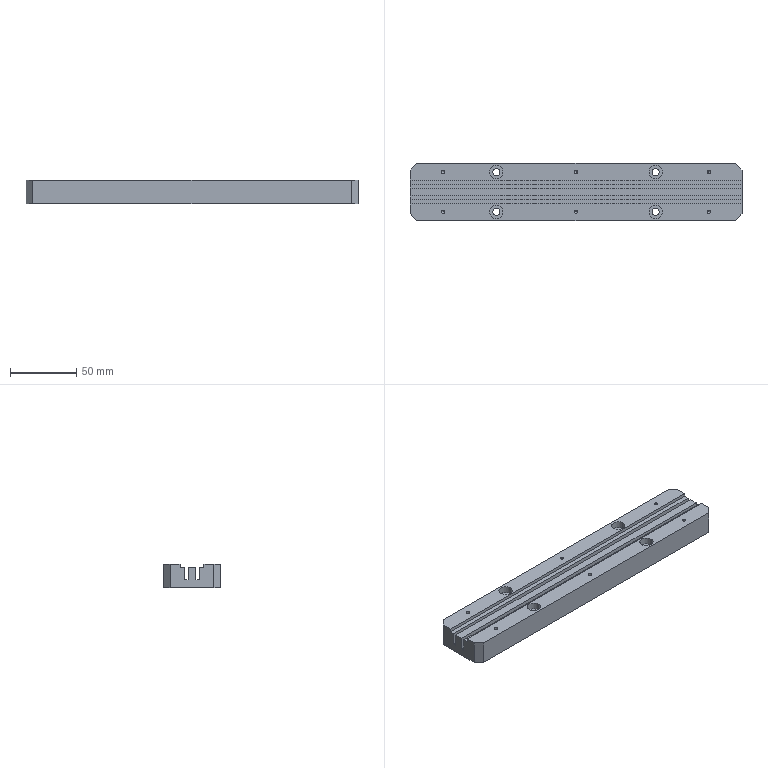Part | STEP file | D01 | 1 solid | 66 faces | box 250 x 43 x 18 mm | volume 165403 mm3 | cylinder 28 | plane 26 | cone 12 | commonest cylinder face diameters 2.5 x12 5.5 x8 10 x8